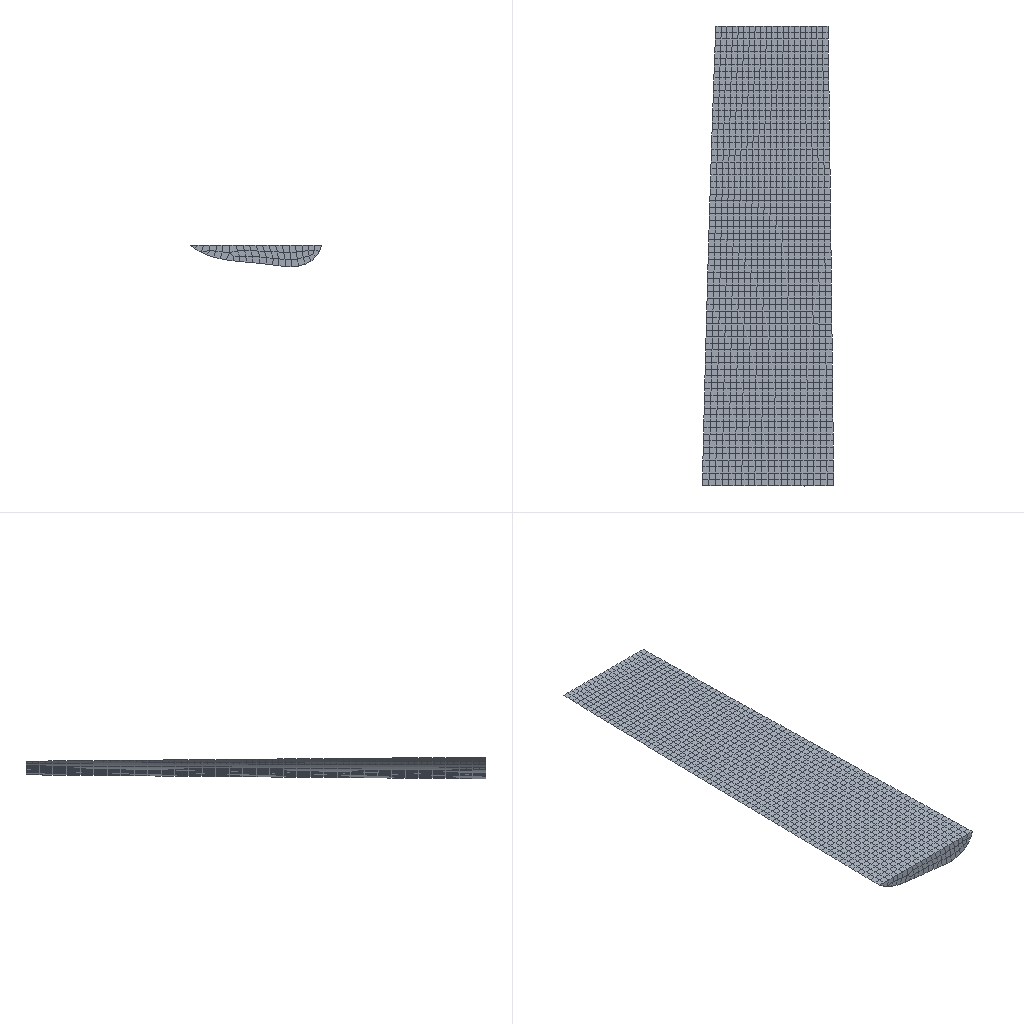Simulation study | ansys workbench
Set-up summary:
category,name,step,type,value,unit,region
solver,ansys_workbench
units,mm-N-s-tonne (MPa),,stated,"/units,MPA"
analysis,deck-1/LS1,,static
load_step,deck-1/LS1,deck-1/LS1,static,nsubst=1; time=1
analysis,deck-2/LS1,,static
load_step,deck-2/LS1,deck-2/LS1,static,nsubst=1; time=1
mesh,deck-1.dat,,nodes,19367
mesh,deck-1.dat,,elements,5254
element_type,SOLID186,,,3692,,deck-1.dat
element_type,SURF154,,,1562,,deck-1.dat
mesh,deck-2.dat,,nodes,22740
mesh,deck-2.dat,,elements,16560
element_type,SOLID187,,,12239,,deck-2.dat
element_type,SURF154,,,4321,,deck-2.dat
material,Structural Steel,,E,200000,tonne s^-2 mm^-1
material,Structural Steel,,nu,0.3
material,Structural Steel,,density,7.85e-09,tonne mm^-3
material,Structural Steel,,conductivity,60.5,tonne mm s^-3 C^-1
material,Structural Steel,,specific_heat,4.34e+08,mm^2 s^-2 C^-1
material,Structural Steel,,cte,1.2e-05,C^-1
material,Structural Steel,,permeability,10000
material,Structural Steel,,resistivity,0.00017,ohm mm
load,Define Force Using Surface Effect Elements,deck-1/LS1,surface-effect pres face 1,-204.694,,SURF154 #2
load,Define Force Using Surface Effect Elements,deck-2/LS1,surface-effect pres face 1,195.599,,SURF154 #2
bc,Fixed Supports,deck-1/model,fixed,[dofs=ALL],,_FIXEDSU
bc,Fixed Supports,deck-2/model,fixed,[dofs=ALL],,_FIXEDSU
named_set,_FIXEDSU,,node,197
named_set,_FIXEDSU,,node,200
Results summary:
result,analyses[0].index,,,1
result,analyses[0].system,,,SYS
result,analyses[0].deck,,,deck-1.dat
result,analyses[0].solve_status,,,completed
result,analyses[0].analysis_type,,,static
result,analyses[0].physics,,,mechanical
result,analyses[0].unit_system,,,"NMM: mm, ton, N, s, mV, mA, degC"
result,analyses[0].n_sets,,,1
result,analyses[0].load_steps[0].set,set=1,,1
result,analyses[0].load_steps[0].time_or_freq,set=1,,1
result,analyses[0].load_steps[0].max_displacement_magnitude,set=1,,120.74
result,analyses[0].load_steps[0].max_von_mises_nodal,set=1,,147216
result,analyses[0].load_steps[0].reaction_force_sum_xyz[1],set=1,,289000
result,analyses[0].load_steps[0].reaction_force_sum_xyz[2],set=1,,-0.001171
result,analyses[0].load_steps[0].reaction_force_sum_xyz[3],set=1,,-0.0007334
result,analyses[1].index,,,2
result,analyses[1].system,,,SYS-1
result,analyses[1].deck,,,deck-2.dat
result,analyses[1].solve_status,,,completed
result,analyses[1].analysis_type,,,static
result,analyses[1].physics,,,mechanical
result,analyses[1].unit_system,,,"NMM: mm, ton, N, s, mV, mA, degC"
result,analyses[1].n_sets,,,1
result,analyses[1].load_steps[0].set,set=1,,1
result,analyses[1].load_steps[0].time_or_freq,set=1,,1
result,analyses[1].load_steps[0].max_displacement_magnitude,set=1,,248.575
result,analyses[1].load_steps[0].max_von_mises_nodal,set=1,,525254
result,analyses[1].load_steps[0].reaction_force_sum_xyz[1],set=1,,-288988
result,analyses[1].load_steps[0].reaction_force_sum_xyz[2],set=1,,0.0001331
result,analyses[1].load_steps[0].reaction_force_sum_xyz[3],set=1,,0.001137